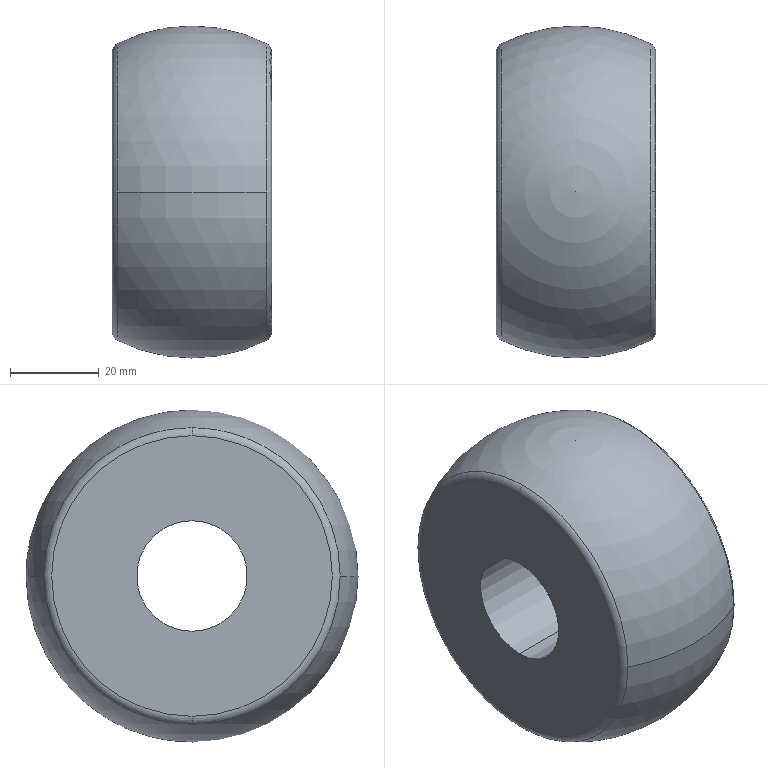Part | STEP file | SceondCKH75wheel | 1 solid | 10 faces | box 36 x 75 x 75 mm | volume 129056 mm3 | torus 4 | sphere 2 | cylinder 2 | plane 2 | commonest cylinder face diameters 25 x2
STEP:
#1=CARTESIAN_POINT('',(-16.901,33.475,0.));
#2=VERTEX_POINT('',#1);
#3=CARTESIAN_POINT('',(-16.901,0.,-33.475));
#4=VERTEX_POINT('',#3);
#5=CARTESIAN_POINT('',(-16.901,0.,0.));
#6=DIRECTION('',(-1.,0.,0.));
#7=DIRECTION('',(0.,0.,1.));
#8=AXIS2_PLACEMENT_3D('',#5,#6,#7);
#9=CIRCLE('',#8,33.475);
#10=EDGE_CURVE('',#2,#4,#9,.T.);
#11=ORIENTED_EDGE('',*,*,#10,.T.);
#12=CARTESIAN_POINT('',(-18.,0.,-31.69));
#13=VERTEX_POINT('',#12);
#14=CARTESIAN_POINT('',(-16.,0.,-31.69));
#15=DIRECTION('',(0.,1.,0.));
#16=DIRECTION('',(0.,0.,1.));
#17=AXIS2_PLACEMENT_3D('',#14,#15,#16);
#18=CIRCLE('',#17,2.);
#19=EDGE_CURVE('',#4,#13,#18,.T.);
#20=ORIENTED_EDGE('',*,*,#19,.T.);
#21=CARTESIAN_POINT('',(-18.,0.,31.69));
#22=VERTEX_POINT('',#21);
#23=CARTESIAN_POINT('',(-18.,0.,0.));
#24=DIRECTION('',(-1.,0.,0.));
#25=DIRECTION('',(0.,0.,1.));
#26=AXIS2_PLACEMENT_3D('',#23,#24,#25);
#27=CIRCLE('',#26,31.69);
#28=EDGE_CURVE('',#22,#13,#27,.T.);
#29=ORIENTED_EDGE('',*,*,#28,.F.);
#30=CARTESIAN_POINT('',(-16.901,0.,33.475));
#31=VERTEX_POINT('',#30);
#32=CARTESIAN_POINT('',(-16.,0.,31.69));
#33=DIRECTION('',(0.,-1.,0.));
#34=DIRECTION('',(0.,0.,-1.));
#35=AXIS2_PLACEMENT_3D('',#32,#33,#34);
#36=CIRCLE('',#35,2.);
#37=EDGE_CURVE('',#31,#22,#36,.T.);
#38=ORIENTED_EDGE('',*,*,#37,.F.);
#39=CARTESIAN_POINT('',(-16.901,0.,0.));
#40=DIRECTION('',(-1.,0.,0.));
#41=DIRECTION('',(0.,0.,1.));
#42=AXIS2_PLACEMENT_3D('',#39,#40,#41);
#43=CIRCLE('',#42,33.475);
#44=EDGE_CURVE('',#31,#2,#43,.T.);
#45=ORIENTED_EDGE('',*,*,#44,.T.);
#46=EDGE_LOOP('',(#11,#20,#29,#38,#45));
#47=FACE_OUTER_BOUND('',#46,.T.);
#48=CARTESIAN_POINT('',(-16.,0.,0.));
#49=DIRECTION('',(-1.,0.,0.));
#50=DIRECTION('',(0.,0.,1.));
#51=AXIS2_PLACEMENT_3D('',#48,#49,#50);
#52=TOROIDAL_SURFACE('',#51,31.69,2.);
#53=ADVANCED_FACE('',(#47),#52,.T.);
#54=CARTESIAN_POINT('',(16.901,0.,-33.475));
#55=VERTEX_POINT('',#54);
#56=CARTESIAN_POINT('',(16.901,-33.475,0.));
#57=VERTEX_POINT('',#56);
#58=CARTESIAN_POINT('',(16.901,0.,0.));
#59=DIRECTION('',(-1.,0.,0.));
#60=DIRECTION('',(0.,0.,1.));
#61=AXIS2_PLACEMENT_3D('',#58,#59,#60);
#62=CIRCLE('',#61,33.475);
#63=EDGE_CURVE('',#55,#57,#62,.T.);
#64=ORIENTED_EDGE('',*,*,#63,.T.);
#65=CARTESIAN_POINT('',(-16.901,-33.475,0.));
#66=VERTEX_POINT('',#65);
#67=CARTESIAN_POINT('',(0.,0.,0.));
#68=DIRECTION('',(0.,0.,-1.));
#69=DIRECTION('',(0.,1.,0.));
#70=AXIS2_PLACEMENT_3D('',#67,#68,#69);
#71=CIRCLE('',#70,37.5);
#72=EDGE_CURVE('',#57,#66,#71,.T.);
#73=ORIENTED_EDGE('',*,*,#72,.T.);
#74=CARTESIAN_POINT('',(-16.901,0.,0.));
#75=DIRECTION('',(-1.,0.,0.));
#76=DIRECTION('',(0.,0.,1.));
#77=AXIS2_PLACEMENT_3D('',#74,#75,#76);
#78=CIRCLE('',#77,33.475);
#79=EDGE_CURVE('',#4,#66,#78,.T.);
#80=ORIENTED_EDGE('',*,*,#79,.F.);
#81=ORIENTED_EDGE('',*,*,#10,.F.);
#82=CARTESIAN_POINT('',(16.901,33.475,0.));
#83=VERTEX_POINT('',#82);
#84=CARTESIAN_POINT('',(0.,0.,0.));
#85=DIRECTION('',(0.,0.,1.));
#86=DIRECTION('',(1.,0.,0.));
#87=AXIS2_PLACEMENT_3D('',#84,#85,#86);
#88=CIRCLE('',#87,37.5);
#89=EDGE_CURVE('',#83,#2,#88,.T.);
#90=ORIENTED_EDGE('',*,*,#89,.F.);
#91=CARTESIAN_POINT('',(16.901,0.,0.));
#92=DIRECTION('',(-1.,0.,0.));
#93=DIRECTION('',(0.,0.,1.));
#94=AXIS2_PLACEMENT_3D('',#91,#92,#93);
#95=CIRCLE('',#94,33.475);
#96=EDGE_CURVE('',#83,#55,#95,.T.);
#97=ORIENTED_EDGE('',*,*,#96,.T.);
#98=EDGE_LOOP('',(#64,#73,#80,#81,#90,#97));
#99=FACE_OUTER_BOUND('',#98,.T.);
#100=CARTESIAN_POINT('',(0.,0.,0.));
#101=DIRECTION('',(0.,0.,-1.));
#102=DIRECTION('',(0.,1.,0.));
#103=AXIS2_PLACEMENT_3D('',#100,#101,#102);
#104=SPHERICAL_SURFACE('',#103,37.5);
#105=ADVANCED_FACE('',(#99),#104,.T.);
#106=CARTESIAN_POINT('',(18.,0.,31.69));
#107=VERTEX_POINT('',#106);
#108=CARTESIAN_POINT('',(18.,0.,-31.69));
#109=VERTEX_POINT('',#108);
#110=CARTESIAN_POINT('',(18.,0.,0.));
#111=DIRECTION('',(-1.,0.,0.));
#112=DIRECTION('',(0.,0.,1.));
#113=AXIS2_PLACEMENT_3D('',#110,#111,#112);
#114=CIRCLE('',#113,31.69);
#115=EDGE_CURVE('',#107,#109,#114,.T.);
#116=ORIENTED_EDGE('',*,*,#115,.T.);
#117=CARTESIAN_POINT('',(16.,0.,-31.69));
#118=DIRECTION('',(0.,1.,0.));
#119=DIRECTION('',(0.,0.,1.));
#120=AXIS2_PLACEMENT_3D('',#117,#118,#119);
#121=CIRCLE('',#120,2.);
#122=EDGE_CURVE('',#109,#55,#121,.T.);
#123=ORIENTED_EDGE('',*,*,#122,.T.);
#124=ORIENTED_EDGE('',*,*,#96,.F.);
#125=CARTESIAN_POINT('',(16.901,0.,33.475));
#126=VERTEX_POINT('',#125);
#127=CARTESIAN_POINT('',(16.901,0.,0.));
#128=DIRECTION('',(-1.,0.,0.));
#129=DIRECTION('',(0.,0.,1.));
#130=AXIS2_PLACEMENT_3D('',#127,#128,#129);
#131=CIRCLE('',#130,33.475);
#132=EDGE_CURVE('',#126,#83,#131,.T.);
#133=ORIENTED_EDGE('',*,*,#132,.F.);
#134=CARTESIAN_POINT('',(16.,0.,31.69));
#135=DIRECTION('',(0.,-1.,0.));
#136=DIRECTION('',(0.,0.,-1.));
#137=AXIS2_PLACEMENT_3D('',#134,#135,#136);
#138=CIRCLE('',#137,2.);
#139=EDGE_CURVE('',#107,#126,#138,.T.);
#140=ORIENTED_EDGE('',*,*,#139,.F.);
#141=EDGE_LOOP('',(#116,#123,#124,#133,#140));
#142=FACE_OUTER_BOUND('',#141,.T.);
#143=CARTESIAN_POINT('',(16.,0.,0.));
#144=DIRECTION('',(-1.,0.,0.));
#145=DIRECTION('',(0.,0.,1.));
#146=AXIS2_PLACEMENT_3D('',#143,#144,#145);
#147=TOROIDAL_SURFACE('',#146,31.69,2.);
#148=ADVANCED_FACE('',(#142),#147,.T.);
#149=CARTESIAN_POINT('',(18.,0.,-12.5));
#150=VERTEX_POINT('',#149);
#151=CARTESIAN_POINT('',(18.,0.,12.5));
#152=VERTEX_POINT('',#151);
#153=CARTESIAN_POINT('',(18.,0.,0.));
#154=DIRECTION('',(-1.,0.,0.));
#155=DIRECTION('',(0.,0.,1.));
#156=AXIS2_PLACEMENT_3D('',#153,#154,#155);
#157=CIRCLE('',#156,12.5);
#158=EDGE_CURVE('',#150,#152,#157,.T.);
#159=ORIENTED_EDGE('',*,*,#158,.F.);
#160=CARTESIAN_POINT('',(-18.,0.,-12.5));
#161=VERTEX_POINT('',#160);
#162=CARTESIAN_POINT('',(50.,0.,-12.5));
#163=DIRECTION('',(-1.,0.,0.));
#164=VECTOR('',#163,1000.);
#165=LINE('',#162,#164);
#166=EDGE_CURVE('',#150,#161,#165,.T.);
#167=ORIENTED_EDGE('',*,*,#166,.T.);
#168=CARTESIAN_POINT('',(-18.,0.,12.5));
#169=VERTEX_POINT('',#168);
#170=CARTESIAN_POINT('',(-18.,0.,0.));
#171=DIRECTION('',(-1.,0.,0.));
#172=DIRECTION('',(0.,0.,1.));
#173=AXIS2_PLACEMENT_3D('',#170,#171,#172);
#174=CIRCLE('',#173,12.5);
#175=EDGE_CURVE('',#161,#169,#174,.T.);
#176=ORIENTED_EDGE('',*,*,#175,.T.);
#177=CARTESIAN_POINT('',(50.,0.,12.5));
#178=DIRECTION('',(-1.,0.,0.));
#179=VECTOR('',#178,1000.);
#180=LINE('',#177,#179);
#181=EDGE_CURVE('',#152,#169,#180,.T.);
#182=ORIENTED_EDGE('',*,*,#181,.F.);
#183=EDGE_LOOP('',(#159,#167,#176,#182));
#184=FACE_OUTER_BOUND('',#183,.T.);
#185=CARTESIAN_POINT('',(50.,0.,0.));
#186=DIRECTION('',(-1.,0.,0.));
#187=DIRECTION('',(0.,0.,1.));
#188=AXIS2_PLACEMENT_3D('',#185,#186,#187);
#189=CYLINDRICAL_SURFACE('',#188,12.5);
#190=ADVANCED_FACE('',(#184),#189,.F.);
#191=CARTESIAN_POINT('',(-18.,0.,0.));
#192=DIRECTION('',(-1.,0.,0.));
#193=DIRECTION('',(0.,0.,1.));
#194=AXIS2_PLACEMENT_3D('',#191,#192,#193);
#195=CIRCLE('',#194,12.5);
#196=EDGE_CURVE('',#169,#161,#195,.T.);
#197=ORIENTED_EDGE('',*,*,#196,.F.);
#198=ORIENTED_EDGE('',*,*,#175,.F.);
#199=EDGE_LOOP('',(#197,#198));
#200=FACE_BOUND('',#199,.T.);
#201=ORIENTED_EDGE('',*,*,#28,.T.);
#202=CARTESIAN_POINT('',(-18.,0.,0.));
#203=DIRECTION('',(-1.,0.,0.));
#204=DIRECTION('',(0.,0.,1.));
#205=AXIS2_PLACEMENT_3D('',#202,#203,#204);
#206=CIRCLE('',#205,31.69);
#207=EDGE_CURVE('',#13,#22,#206,.T.);
#208=ORIENTED_EDGE('',*,*,#207,.T.);
#209=EDGE_LOOP('',(#201,#208));
#210=FACE_OUTER_BOUND('',#209,.T.);
#211=CARTESIAN_POINT('',(-18.,31.69,0.));
#212=DIRECTION('',(1.,0.,0.));
#213=DIRECTION('',(0.,0.,-1.));
#214=AXIS2_PLACEMENT_3D('',#211,#212,#213);
#215=PLANE('',#214);
#216=ADVANCED_FACE('',(#200,#210),#215,.F.);
#217=ORIENTED_EDGE('',*,*,#166,.F.);
#218=CARTESIAN_POINT('',(18.,0.,0.));
#219=DIRECTION('',(-1.,0.,0.));
#220=DIRECTION('',(0.,0.,1.));
#221=AXIS2_PLACEMENT_3D('',#218,#219,#220);
#222=CIRCLE('',#221,12.5);
#223=EDGE_CURVE('',#152,#150,#222,.T.);
#224=ORIENTED_EDGE('',*,*,#223,.F.);
#225=ORIENTED_EDGE('',*,*,#181,.T.);
#226=ORIENTED_EDGE('',*,*,#196,.T.);
#227=EDGE_LOOP('',(#217,#224,#225,#226));
#228=FACE_OUTER_BOUND('',#227,.T.);
#229=CARTESIAN_POINT('',(50.,0.,0.));
#230=DIRECTION('',(-1.,0.,0.));
#231=DIRECTION('',(0.,0.,1.));
#232=AXIS2_PLACEMENT_3D('',#229,#230,#231);
#233=CYLINDRICAL_SURFACE('',#232,12.5);
#234=ADVANCED_FACE('',(#228),#233,.F.);
#235=ORIENTED_EDGE('',*,*,#115,.F.);
#236=CARTESIAN_POINT('',(18.,0.,0.));
#237=DIRECTION('',(-1.,0.,0.));
#238=DIRECTION('',(0.,0.,1.));
#239=AXIS2_PLACEMENT_3D('',#236,#237,#238);
#240=CIRCLE('',#239,31.69);
#241=EDGE_CURVE('',#109,#107,#240,.T.);
#242=ORIENTED_EDGE('',*,*,#241,.F.);
#243=EDGE_LOOP('',(#235,#242));
#244=FACE_OUTER_BOUND('',#243,.T.);
#245=ORIENTED_EDGE('',*,*,#223,.T.);
#246=ORIENTED_EDGE('',*,*,#158,.T.);
#247=EDGE_LOOP('',(#245,#246));
#248=FACE_BOUND('',#247,.T.);
#249=CARTESIAN_POINT('',(18.,12.5,0.));
#250=DIRECTION('',(-1.,0.,0.));
#251=DIRECTION('',(0.,0.,1.));
#252=AXIS2_PLACEMENT_3D('',#249,#250,#251);
#253=PLANE('',#252);
#254=ADVANCED_FACE('',(#244,#248),#253,.F.);
#255=ORIENTED_EDGE('',*,*,#122,.F.);
#256=ORIENTED_EDGE('',*,*,#241,.T.);
#257=ORIENTED_EDGE('',*,*,#139,.T.);
#258=CARTESIAN_POINT('',(16.901,0.,0.));
#259=DIRECTION('',(-1.,0.,0.));
#260=DIRECTION('',(0.,0.,1.));
#261=AXIS2_PLACEMENT_3D('',#258,#259,#260);
#262=CIRCLE('',#261,33.475);
#263=EDGE_CURVE('',#57,#126,#262,.T.);
#264=ORIENTED_EDGE('',*,*,#263,.F.);
#265=ORIENTED_EDGE('',*,*,#63,.F.);
#266=EDGE_LOOP('',(#255,#256,#257,#264,#265));
#267=FACE_OUTER_BOUND('',#266,.T.);
#268=CARTESIAN_POINT('',(16.,0.,0.));
#269=DIRECTION('',(-1.,0.,0.));
#270=DIRECTION('',(0.,0.,1.));
#271=AXIS2_PLACEMENT_3D('',#268,#269,#270);
#272=TOROIDAL_SURFACE('',#271,31.69,2.);
#273=ADVANCED_FACE('',(#267),#272,.T.);
#274=ORIENTED_EDGE('',*,*,#72,.F.);
#275=ORIENTED_EDGE('',*,*,#263,.T.);
#276=ORIENTED_EDGE('',*,*,#132,.T.);
#277=ORIENTED_EDGE('',*,*,#89,.T.);
#278=ORIENTED_EDGE('',*,*,#44,.F.);
#279=CARTESIAN_POINT('',(-16.901,0.,0.));
#280=DIRECTION('',(-1.,0.,0.));
#281=DIRECTION('',(0.,0.,1.));
#282=AXIS2_PLACEMENT_3D('',#279,#280,#281);
#283=CIRCLE('',#282,33.475);
#284=EDGE_CURVE('',#66,#31,#283,.T.);
#285=ORIENTED_EDGE('',*,*,#284,.F.);
#286=EDGE_LOOP('',(#274,#275,#276,#277,#278,#285));
#287=FACE_OUTER_BOUND('',#286,.T.);
#288=CARTESIAN_POINT('',(0.,0.,0.));
#289=DIRECTION('',(0.,0.,-1.));
#290=DIRECTION('',(0.,1.,0.));
#291=AXIS2_PLACEMENT_3D('',#288,#289,#290);
#292=SPHERICAL_SURFACE('',#291,37.5);
#293=ADVANCED_FACE('',(#287),#292,.T.);
#294=ORIENTED_EDGE('',*,*,#19,.F.);
#295=ORIENTED_EDGE('',*,*,#79,.T.);
#296=ORIENTED_EDGE('',*,*,#284,.T.);
#297=ORIENTED_EDGE('',*,*,#37,.T.);
#298=ORIENTED_EDGE('',*,*,#207,.F.);
#299=EDGE_LOOP('',(#294,#295,#296,#297,#298));
#300=FACE_OUTER_BOUND('',#299,.T.);
#301=CARTESIAN_POINT('',(-16.,0.,0.));
#302=DIRECTION('',(-1.,0.,0.));
#303=DIRECTION('',(0.,0.,1.));
#304=AXIS2_PLACEMENT_3D('',#301,#302,#303);
#305=TOROIDAL_SURFACE('',#304,31.69,2.);
#306=ADVANCED_FACE('',(#300),#305,.T.);
#307=CLOSED_SHELL('',(#53,#105,#148,#190,#216,#234,#254,#273,#293,#306));
#308=MANIFOLD_SOLID_BREP('',#307);
#309=CARTESIAN_POINT('',(0.,0.,0.));
#310=DIRECTION('',(0.,0.,1.));
#311=DIRECTION('',(1.,0.,0.));
#312=AXIS2_PLACEMENT_3D('',#309,#310,#311);
#313=(LENGTH_UNIT()NAMED_UNIT(*)SI_UNIT(.MILLI.,.METRE.));
#314=UNCERTAINTY_MEASURE_WITH_UNIT(LENGTH_MEASURE(0.00001),#313,'','');
#315=(NAMED_UNIT(*)PLANE_ANGLE_UNIT()SI_UNIT($,.RADIAN.));
#316=(NAMED_UNIT(*)SI_UNIT($,.STERADIAN.)SOLID_ANGLE_UNIT());
#317=(GEOMETRIC_REPRESENTATION_CONTEXT(3)GLOBAL_UNCERTAINTY_ASSIGNED_CONTEXT((#314))GLOBAL_UNIT_ASSIGNED_CONTEXT((#313,#315,#316))REPRESENTATION_CONTEXT('',''));
#318=ADVANCED_BREP_SHAPE_REPRESENTATION('',(#308,#312),#317);